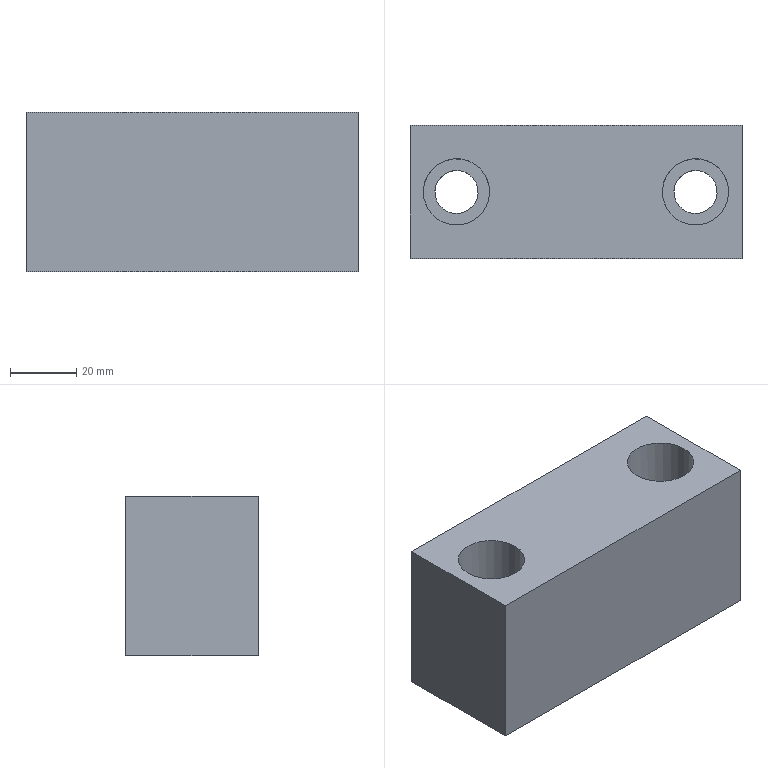Part | STEP file | gslz 2016.10.28-13_id774_x_t | 1 solid | 12 faces | box 100 x 40 x 48 mm | volume 169823 mm3 | plane 8 | cylinder 4 | commonest cylinder face diameters 13 x2 20 x2
STEP:
#1=CARTESIAN_POINT('',(0.,0.,0.));
#2=DIRECTION('',(0.,0.,1.));
#3=DIRECTION('',(1.,0.,0.));
#4=AXIS2_PLACEMENT_3D('',#1,#2,#3);
#5=CARTESIAN_POINT('',(-1056.695,-13.439,0.));
#6=VERTEX_POINT('',#5);
#7=CARTESIAN_POINT('',(-1156.695,-13.439,0.));
#8=VERTEX_POINT('',#7);
#9=CARTESIAN_POINT('',(-1172.695,-13.439,0.));
#10=DIRECTION('',(-1.,0.,0.));
#11=VECTOR('',#10,1.);
#12=LINE('',#9,#11);
#13=CARTESIAN_POINT('',(-1056.695,-13.439,-43.));
#14=DIRECTION('',(0.,1.,0.));
#15=DIRECTION('',(-1.,0.,0.));
#16=AXIS2_PLACEMENT_3D('',#13,#14,#15);
#17=PLANE('',#16);
#18=CARTESIAN_POINT('',(116.,43.));
#19=DIRECTION('',(1.,0.));
#20=VECTOR('',#19,1.);
#21=LINE('',#18,#20);
#22=(GEOMETRIC_REPRESENTATION_CONTEXT(2)PARAMETRIC_REPRESENTATION_CONTEXT()REPRESENTATION_CONTEXT('',''));
#23=DEFINITIONAL_REPRESENTATION('',(#21),#22);
#24=PCURVE('',#17,#23);
#25=CARTESIAN_POINT('',(-1172.695,-123.667,0.));
#26=DIRECTION('',(0.,0.,1.));
#27=DIRECTION('',(-1.,0.,0.));
#28=AXIS2_PLACEMENT_3D('',#25,#26,#27);
#29=PLANE('',#28);
#30=CARTESIAN_POINT('',(0.,-110.228));
#31=DIRECTION('',(1.,0.));
#32=VECTOR('',#31,1.);
#33=LINE('',#30,#32);
#34=(GEOMETRIC_REPRESENTATION_CONTEXT(2)PARAMETRIC_REPRESENTATION_CONTEXT()REPRESENTATION_CONTEXT('',''));
#35=DEFINITIONAL_REPRESENTATION('',(#33),#34);
#36=PCURVE('',#29,#35);
#37=SURFACE_CURVE('',#12,(#24,#36),.PCURVE_S1.);
#38=EDGE_CURVE('',#6,#8,#37,.T.);
#39=ORIENTED_EDGE('',*,*,#38,.F.);
#40=CARTESIAN_POINT('',(-1056.695,-13.439,-48.));
#41=VERTEX_POINT('',#40);
#42=CARTESIAN_POINT('',(-1056.695,-13.439,-43.));
#43=DIRECTION('',(0.,0.,1.));
#44=VECTOR('',#43,1.);
#45=LINE('',#42,#44);
#46=CARTESIAN_POINT('',(0.,0.));
#47=DIRECTION('',(0.,1.));
#48=VECTOR('',#47,1.);
#49=LINE('',#46,#48);
#50=(GEOMETRIC_REPRESENTATION_CONTEXT(2)PARAMETRIC_REPRESENTATION_CONTEXT()REPRESENTATION_CONTEXT('',''));
#51=DEFINITIONAL_REPRESENTATION('',(#49),#50);
#52=PCURVE('',#17,#51);
#53=CARTESIAN_POINT('',(-1056.695,-214.939,-43.));
#54=DIRECTION('',(1.,0.,0.));
#55=DIRECTION('',(0.,0.,1.));
#56=AXIS2_PLACEMENT_3D('',#53,#54,#55);
#57=PLANE('',#56);
#58=CARTESIAN_POINT('',(0.,-201.5));
#59=DIRECTION('',(1.,0.));
#60=VECTOR('',#59,1.);
#61=LINE('',#58,#60);
#62=(GEOMETRIC_REPRESENTATION_CONTEXT(2)PARAMETRIC_REPRESENTATION_CONTEXT()REPRESENTATION_CONTEXT('',''));
#63=DEFINITIONAL_REPRESENTATION('',(#61),#62);
#64=PCURVE('',#57,#63);
#65=SURFACE_CURVE('',#45,(#52,#64),.PCURVE_S1.);
#66=EDGE_CURVE('',#41,#6,#65,.T.);
#67=ORIENTED_EDGE('',*,*,#66,.F.);
#68=CARTESIAN_POINT('',(-1156.695,-13.439,-48.));
#69=VERTEX_POINT('',#68);
#70=CARTESIAN_POINT('',(-1119.195,-13.439,-48.));
#71=DIRECTION('',(-1.,0.,0.));
#72=VECTOR('',#71,1.);
#73=LINE('',#70,#72);
#74=CARTESIAN_POINT('',(62.5,-5.));
#75=DIRECTION('',(1.,0.));
#76=VECTOR('',#75,1.);
#77=LINE('',#74,#76);
#78=(GEOMETRIC_REPRESENTATION_CONTEXT(2)PARAMETRIC_REPRESENTATION_CONTEXT()REPRESENTATION_CONTEXT('',''));
#79=DEFINITIONAL_REPRESENTATION('',(#77),#78);
#80=PCURVE('',#17,#79);
#81=CARTESIAN_POINT('',(-1119.195,-219.939,-48.));
#82=DIRECTION('',(0.,0.,1.));
#83=DIRECTION('',(-1.,0.,0.));
#84=AXIS2_PLACEMENT_3D('',#81,#82,#83);
#85=PLANE('',#84);
#86=CARTESIAN_POINT('',(0.,-206.5));
#87=DIRECTION('',(1.,0.));
#88=VECTOR('',#87,1.);
#89=LINE('',#86,#88);
#90=(GEOMETRIC_REPRESENTATION_CONTEXT(2)PARAMETRIC_REPRESENTATION_CONTEXT()REPRESENTATION_CONTEXT('',''));
#91=DEFINITIONAL_REPRESENTATION('',(#89),#90);
#92=PCURVE('',#85,#91);
#93=SURFACE_CURVE('',#73,(#80,#92),.PCURVE_S1.);
#94=EDGE_CURVE('',#41,#69,#93,.T.);
#95=ORIENTED_EDGE('',*,*,#94,.T.);
#96=CARTESIAN_POINT('',(-1156.695,-13.439,-43.));
#97=DIRECTION('',(0.,0.,1.));
#98=VECTOR('',#97,1.);
#99=LINE('',#96,#98);
#100=CARTESIAN_POINT('',(100.,0.));
#101=DIRECTION('',(0.,1.));
#102=VECTOR('',#101,1.);
#103=LINE('',#100,#102);
#104=(GEOMETRIC_REPRESENTATION_CONTEXT(2)PARAMETRIC_REPRESENTATION_CONTEXT()REPRESENTATION_CONTEXT('',''));
#105=DEFINITIONAL_REPRESENTATION('',(#103),#104);
#106=PCURVE('',#17,#105);
#107=CARTESIAN_POINT('',(-1156.695,-24.939,-43.));
#108=DIRECTION('',(-1.,0.,0.));
#109=DIRECTION('',(0.,-1.,0.));
#110=AXIS2_PLACEMENT_3D('',#107,#108,#109);
#111=PLANE('',#110);
#112=CARTESIAN_POINT('',(-11.5,0.));
#113=DIRECTION('',(0.,1.));
#114=VECTOR('',#113,1.);
#115=LINE('',#112,#114);
#116=(GEOMETRIC_REPRESENTATION_CONTEXT(2)PARAMETRIC_REPRESENTATION_CONTEXT()REPRESENTATION_CONTEXT('',''));
#117=DEFINITIONAL_REPRESENTATION('',(#115),#116);
#118=PCURVE('',#111,#117);
#119=SURFACE_CURVE('',#99,(#106,#118),.PCURVE_S1.);
#120=EDGE_CURVE('',#69,#8,#119,.T.);
#121=ORIENTED_EDGE('',*,*,#120,.T.);
#122=EDGE_LOOP('',(#39,#67,#95,#121));
#123=FACE_BOUND('',#122,.T.);
#124=ADVANCED_FACE('',(#123),#17,.T.);
#125=CARTESIAN_POINT('',(-1156.695,-53.439,0.));
#126=VERTEX_POINT('',#125);
#127=CARTESIAN_POINT('',(-1156.695,-24.939,0.));
#128=DIRECTION('',(0.,-1.,0.));
#129=VECTOR('',#128,1.);
#130=LINE('',#127,#129);
#131=CARTESIAN_POINT('',(0.,43.));
#132=DIRECTION('',(1.,0.));
#133=VECTOR('',#132,1.);
#134=LINE('',#131,#133);
#135=(GEOMETRIC_REPRESENTATION_CONTEXT(2)PARAMETRIC_REPRESENTATION_CONTEXT()REPRESENTATION_CONTEXT('',''));
#136=DEFINITIONAL_REPRESENTATION('',(#134),#135);
#137=PCURVE('',#111,#136);
#138=CARTESIAN_POINT('',(-16.,-98.728));
#139=DIRECTION('',(0.,1.));
#140=VECTOR('',#139,1.);
#141=LINE('',#138,#140);
#142=(GEOMETRIC_REPRESENTATION_CONTEXT(2)PARAMETRIC_REPRESENTATION_CONTEXT()REPRESENTATION_CONTEXT('',''));
#143=DEFINITIONAL_REPRESENTATION('',(#141),#142);
#144=PCURVE('',#29,#143);
#145=SURFACE_CURVE('',#130,(#137,#144),.PCURVE_S1.);
#146=EDGE_CURVE('',#8,#126,#145,.T.);
#147=ORIENTED_EDGE('',*,*,#146,.F.);
#148=ORIENTED_EDGE('',*,*,#120,.F.);
#149=CARTESIAN_POINT('',(-1156.695,-53.439,-48.));
#150=VERTEX_POINT('',#149);
#151=CARTESIAN_POINT('',(-1156.695,-219.939,-48.));
#152=DIRECTION('',(0.,-1.,0.));
#153=VECTOR('',#152,1.);
#154=LINE('',#151,#153);
#155=CARTESIAN_POINT('',(195.,-5.));
#156=DIRECTION('',(1.,0.));
#157=VECTOR('',#156,1.);
#158=LINE('',#155,#157);
#159=(GEOMETRIC_REPRESENTATION_CONTEXT(2)PARAMETRIC_REPRESENTATION_CONTEXT()REPRESENTATION_CONTEXT('',''));
#160=DEFINITIONAL_REPRESENTATION('',(#158),#159);
#161=PCURVE('',#111,#160);
#162=CARTESIAN_POINT('',(37.5,0.));
#163=DIRECTION('',(0.,1.));
#164=VECTOR('',#163,1.);
#165=LINE('',#162,#164);
#166=(GEOMETRIC_REPRESENTATION_CONTEXT(2)PARAMETRIC_REPRESENTATION_CONTEXT()REPRESENTATION_CONTEXT('',''));
#167=DEFINITIONAL_REPRESENTATION('',(#165),#166);
#168=PCURVE('',#85,#167);
#169=SURFACE_CURVE('',#154,(#161,#168),.PCURVE_S1.);
#170=EDGE_CURVE('',#69,#150,#169,.T.);
#171=ORIENTED_EDGE('',*,*,#170,.T.);
#172=CARTESIAN_POINT('',(-1156.695,-53.439,-25.5));
#173=DIRECTION('',(0.,0.,-1.));
#174=VECTOR('',#173,1.);
#175=LINE('',#172,#174);
#176=CARTESIAN_POINT('',(28.5,17.5));
#177=DIRECTION('',(0.,-1.));
#178=VECTOR('',#177,1.);
#179=LINE('',#176,#178);
#180=(GEOMETRIC_REPRESENTATION_CONTEXT(2)PARAMETRIC_REPRESENTATION_CONTEXT()REPRESENTATION_CONTEXT('',''));
#181=DEFINITIONAL_REPRESENTATION('',(#179),#180);
#182=PCURVE('',#111,#181);
#183=CARTESIAN_POINT('',(-1101.695,-53.439,-25.5));
#184=DIRECTION('',(0.,1.,0.));
#185=DIRECTION('',(0.,0.,-1.));
#186=AXIS2_PLACEMENT_3D('',#183,#184,#185);
#187=PLANE('',#186);
#188=CARTESIAN_POINT('',(0.,55.));
#189=DIRECTION('',(1.,0.));
#190=VECTOR('',#189,1.);
#191=LINE('',#188,#190);
#192=(GEOMETRIC_REPRESENTATION_CONTEXT(2)PARAMETRIC_REPRESENTATION_CONTEXT()REPRESENTATION_CONTEXT('',''));
#193=DEFINITIONAL_REPRESENTATION('',(#191),#192);
#194=PCURVE('',#187,#193);
#195=SURFACE_CURVE('',#175,(#182,#194),.PCURVE_S1.);
#196=EDGE_CURVE('',#126,#150,#195,.T.);
#197=ORIENTED_EDGE('',*,*,#196,.F.);
#198=EDGE_LOOP('',(#147,#148,#171,#197));
#199=FACE_BOUND('',#198,.T.);
#200=ADVANCED_FACE('',(#199),#111,.T.);
#201=ORIENTED_EDGE('',*,*,#196,.T.);
#202=CARTESIAN_POINT('',(-1056.695,-53.439,-48.));
#203=VERTEX_POINT('',#202);
#204=CARTESIAN_POINT('',(-1119.195,-53.439,-48.));
#205=DIRECTION('',(1.,0.,0.));
#206=VECTOR('',#205,1.);
#207=LINE('',#204,#206);
#208=CARTESIAN_POINT('',(22.5,17.5));
#209=DIRECTION('',(0.,-1.));
#210=VECTOR('',#209,1.);
#211=LINE('',#208,#210);
#212=(GEOMETRIC_REPRESENTATION_CONTEXT(2)PARAMETRIC_REPRESENTATION_CONTEXT()REPRESENTATION_CONTEXT('',''));
#213=DEFINITIONAL_REPRESENTATION('',(#211),#212);
#214=PCURVE('',#187,#213);
#215=CARTESIAN_POINT('',(0.,-166.5));
#216=DIRECTION('',(-1.,0.));
#217=VECTOR('',#216,1.);
#218=LINE('',#215,#217);
#219=(GEOMETRIC_REPRESENTATION_CONTEXT(2)PARAMETRIC_REPRESENTATION_CONTEXT()REPRESENTATION_CONTEXT('',''));
#220=DEFINITIONAL_REPRESENTATION('',(#218),#219);
#221=PCURVE('',#85,#220);
#222=SURFACE_CURVE('',#207,(#214,#221),.PCURVE_S1.);
#223=EDGE_CURVE('',#150,#203,#222,.T.);
#224=ORIENTED_EDGE('',*,*,#223,.T.);
#225=CARTESIAN_POINT('',(-1056.695,-53.439,0.));
#226=VERTEX_POINT('',#225);
#227=CARTESIAN_POINT('',(-1056.695,-53.439,-43.));
#228=DIRECTION('',(0.,0.,-1.));
#229=VECTOR('',#228,1.);
#230=LINE('',#227,#229);
#231=CARTESIAN_POINT('',(17.5,-45.));
#232=DIRECTION('',(1.,0.));
#233=VECTOR('',#232,1.);
#234=LINE('',#231,#233);
#235=(GEOMETRIC_REPRESENTATION_CONTEXT(2)PARAMETRIC_REPRESENTATION_CONTEXT()REPRESENTATION_CONTEXT('',''));
#236=DEFINITIONAL_REPRESENTATION('',(#234),#235);
#237=PCURVE('',#187,#236);
#238=CARTESIAN_POINT('',(0.,-161.5));
#239=DIRECTION('',(-1.,0.));
#240=VECTOR('',#239,1.);
#241=LINE('',#238,#240);
#242=(GEOMETRIC_REPRESENTATION_CONTEXT(2)PARAMETRIC_REPRESENTATION_CONTEXT()REPRESENTATION_CONTEXT('',''));
#243=DEFINITIONAL_REPRESENTATION('',(#241),#242);
#244=PCURVE('',#57,#243);
#245=SURFACE_CURVE('',#230,(#237,#244),.PCURVE_S1.);
#246=EDGE_CURVE('',#226,#203,#245,.T.);
#247=ORIENTED_EDGE('',*,*,#246,.F.);
#248=CARTESIAN_POINT('',(-1101.695,-53.439,0.));
#249=DIRECTION('',(-1.,0.,0.));
#250=VECTOR('',#249,1.);
#251=LINE('',#248,#250);
#252=CARTESIAN_POINT('',(-25.5,0.));
#253=DIRECTION('',(0.,1.));
#254=VECTOR('',#253,1.);
#255=LINE('',#252,#254);
#256=(GEOMETRIC_REPRESENTATION_CONTEXT(2)PARAMETRIC_REPRESENTATION_CONTEXT()REPRESENTATION_CONTEXT('',''));
#257=DEFINITIONAL_REPRESENTATION('',(#255),#256);
#258=PCURVE('',#187,#257);
#259=CARTESIAN_POINT('',(-71.,-70.228));
#260=DIRECTION('',(1.,0.));
#261=VECTOR('',#260,1.);
#262=LINE('',#259,#261);
#263=(GEOMETRIC_REPRESENTATION_CONTEXT(2)PARAMETRIC_REPRESENTATION_CONTEXT()REPRESENTATION_CONTEXT('',''));
#264=DEFINITIONAL_REPRESENTATION('',(#262),#263);
#265=PCURVE('',#29,#264);
#266=SURFACE_CURVE('',#251,(#258,#265),.PCURVE_S1.);
#267=EDGE_CURVE('',#226,#126,#266,.T.);
#268=ORIENTED_EDGE('',*,*,#267,.T.);
#269=EDGE_LOOP('',(#201,#224,#247,#268));
#270=FACE_BOUND('',#269,.T.);
#271=ADVANCED_FACE('',(#270),#187,.F.);
#272=ORIENTED_EDGE('',*,*,#246,.T.);
#273=CARTESIAN_POINT('',(-1056.695,-219.939,-48.));
#274=DIRECTION('',(0.,1.,0.));
#275=VECTOR('',#274,1.);
#276=LINE('',#273,#275);
#277=CARTESIAN_POINT('',(-5.,5.));
#278=DIRECTION('',(0.,-1.));
#279=VECTOR('',#278,1.);
#280=LINE('',#277,#279);
#281=(GEOMETRIC_REPRESENTATION_CONTEXT(2)PARAMETRIC_REPRESENTATION_CONTEXT()REPRESENTATION_CONTEXT('',''));
#282=DEFINITIONAL_REPRESENTATION('',(#280),#281);
#283=PCURVE('',#57,#282);
#284=CARTESIAN_POINT('',(-62.5,0.));
#285=DIRECTION('',(0.,-1.));
#286=VECTOR('',#285,1.);
#287=LINE('',#284,#286);
#288=(GEOMETRIC_REPRESENTATION_CONTEXT(2)PARAMETRIC_REPRESENTATION_CONTEXT()REPRESENTATION_CONTEXT('',''));
#289=DEFINITIONAL_REPRESENTATION('',(#287),#288);
#290=PCURVE('',#85,#289);
#291=SURFACE_CURVE('',#276,(#283,#290),.PCURVE_S1.);
#292=EDGE_CURVE('',#203,#41,#291,.T.);
#293=ORIENTED_EDGE('',*,*,#292,.T.);
#294=ORIENTED_EDGE('',*,*,#66,.T.);
#295=CARTESIAN_POINT('',(-1056.695,-214.939,0.));
#296=DIRECTION('',(0.,1.,0.));
#297=VECTOR('',#296,1.);
#298=LINE('',#295,#297);
#299=CARTESIAN_POINT('',(43.,0.));
#300=DIRECTION('',(0.,-1.));
#301=VECTOR('',#300,1.);
#302=LINE('',#299,#301);
#303=(GEOMETRIC_REPRESENTATION_CONTEXT(2)PARAMETRIC_REPRESENTATION_CONTEXT()REPRESENTATION_CONTEXT('',''));
#304=DEFINITIONAL_REPRESENTATION('',(#302),#303);
#305=PCURVE('',#57,#304);
#306=CARTESIAN_POINT('',(-116.,91.272));
#307=DIRECTION('',(0.,-1.));
#308=VECTOR('',#307,1.);
#309=LINE('',#306,#308);
#310=(GEOMETRIC_REPRESENTATION_CONTEXT(2)PARAMETRIC_REPRESENTATION_CONTEXT()REPRESENTATION_CONTEXT('',''));
#311=DEFINITIONAL_REPRESENTATION('',(#309),#310);
#312=PCURVE('',#29,#311);
#313=SURFACE_CURVE('',#298,(#305,#312),.PCURVE_S1.);
#314=EDGE_CURVE('',#226,#6,#313,.T.);
#315=ORIENTED_EDGE('',*,*,#314,.F.);
#316=EDGE_LOOP('',(#272,#293,#294,#315));
#317=FACE_BOUND('',#316,.T.);
#318=ADVANCED_FACE('',(#317),#57,.T.);
#319=CARTESIAN_POINT('',(-1071.786,-39.847,-48.));
#320=VERTEX_POINT('',#319);
#321=CARTESIAN_POINT('',(-1070.695,-33.439,-48.));
#322=DIRECTION('',(0.,0.,1.));
#323=DIRECTION('',(-0.1678,-0.9858,0.));
#324=AXIS2_PLACEMENT_3D('',#321,#322,#323);
#325=CIRCLE('',#324,6.5);
#326=CARTESIAN_POINT('',(-48.5,-186.5));
#327=DIRECTION('',(0.1678,0.9858));
#328=AXIS2_PLACEMENT_2D('',#326,#327);
#329=CIRCLE('',#328,6.5);
#330=(GEOMETRIC_REPRESENTATION_CONTEXT(2)PARAMETRIC_REPRESENTATION_CONTEXT()REPRESENTATION_CONTEXT('',''));
#331=DEFINITIONAL_REPRESENTATION('',(#329),#330);
#332=PCURVE('',#85,#331);
#333=CARTESIAN_POINT('',(-1070.695,-33.439,-8.541));
#334=DIRECTION('',(0.,0.,-1.));
#335=DIRECTION('',(-1.,0.,0.));
#336=AXIS2_PLACEMENT_3D('',#333,#334,#335);
#337=CYLINDRICAL_SURFACE('',#336,6.5);
#338=CARTESIAN_POINT('',(11.164,39.459));
#339=DIRECTION('',(-1.,0.));
#340=VECTOR('',#339,1.);
#341=LINE('',#338,#340);
#342=(GEOMETRIC_REPRESENTATION_CONTEXT(2)PARAMETRIC_REPRESENTATION_CONTEXT()REPRESENTATION_CONTEXT('',''));
#343=DEFINITIONAL_REPRESENTATION('',(#341),#342);
#344=PCURVE('',#337,#343);
#345=SURFACE_CURVE('',#325,(#332,#344),.PCURVE_S1.);
#346=EDGE_CURVE('',#320,#320,#345,.T.);
#347=ORIENTED_EDGE('',*,*,#346,.T.);
#348=EDGE_LOOP('',(#347));
#349=FACE_BOUND('',#348,.T.);
#350=CARTESIAN_POINT('',(-1143.786,-39.847,-48.));
#351=VERTEX_POINT('',#350);
#352=CARTESIAN_POINT('',(-1142.695,-33.439,-48.));
#353=DIRECTION('',(0.,0.,1.));
#354=DIRECTION('',(-0.1678,-0.9858,0.));
#355=AXIS2_PLACEMENT_3D('',#352,#353,#354);
#356=CIRCLE('',#355,6.5);
#357=CARTESIAN_POINT('',(23.5,-186.5));
#358=DIRECTION('',(0.1678,0.9858));
#359=AXIS2_PLACEMENT_2D('',#357,#358);
#360=CIRCLE('',#359,6.5);
#361=(GEOMETRIC_REPRESENTATION_CONTEXT(2)PARAMETRIC_REPRESENTATION_CONTEXT()REPRESENTATION_CONTEXT('',''));
#362=DEFINITIONAL_REPRESENTATION('',(#360),#361);
#363=PCURVE('',#85,#362);
#364=CARTESIAN_POINT('',(-1142.695,-33.439,-8.541));
#365=DIRECTION('',(0.,0.,-1.));
#366=DIRECTION('',(-1.,0.,0.));
#367=AXIS2_PLACEMENT_3D('',#364,#365,#366);
#368=CYLINDRICAL_SURFACE('',#367,6.5);
#369=CARTESIAN_POINT('',(11.164,39.459));
#370=DIRECTION('',(-1.,0.));
#371=VECTOR('',#370,1.);
#372=LINE('',#369,#371);
#373=(GEOMETRIC_REPRESENTATION_CONTEXT(2)PARAMETRIC_REPRESENTATION_CONTEXT()REPRESENTATION_CONTEXT('',''));
#374=DEFINITIONAL_REPRESENTATION('',(#372),#373);
#375=PCURVE('',#368,#374);
#376=SURFACE_CURVE('',#356,(#363,#375),.PCURVE_S1.);
#377=EDGE_CURVE('',#351,#351,#376,.T.);
#378=ORIENTED_EDGE('',*,*,#377,.T.);
#379=EDGE_LOOP('',(#378));
#380=FACE_BOUND('',#379,.T.);
#381=ORIENTED_EDGE('',*,*,#292,.F.);
#382=ORIENTED_EDGE('',*,*,#223,.F.);
#383=ORIENTED_EDGE('',*,*,#170,.F.);
#384=ORIENTED_EDGE('',*,*,#94,.F.);
#385=EDGE_LOOP('',(#381,#382,#383,#384));
#386=FACE_BOUND('',#385,.T.);
#387=ADVANCED_FACE('',(#349,#380,#386),#85,.F.);
#388=CARTESIAN_POINT('',(-1060.695,-33.439,0.));
#389=VERTEX_POINT('',#388);
#390=CARTESIAN_POINT('',(-1072.373,-43.297,0.));
#391=VERTEX_POINT('',#390);
#392=CARTESIAN_POINT('',(-1070.695,-33.439,0.));
#393=DIRECTION('',(0.,0.,1.));
#394=DIRECTION('',(1.,0.,0.));
#395=AXIS2_PLACEMENT_3D('',#392,#393,#394);
#396=CIRCLE('',#395,10.);
#397=CARTESIAN_POINT('',(-102.,-90.228));
#398=DIRECTION('',(-1.,0.));
#399=AXIS2_PLACEMENT_2D('',#397,#398);
#400=CIRCLE('',#399,10.);
#401=(GEOMETRIC_REPRESENTATION_CONTEXT(2)PARAMETRIC_REPRESENTATION_CONTEXT()REPRESENTATION_CONTEXT('',''));
#402=DEFINITIONAL_REPRESENTATION('',(#400),#401);
#403=PCURVE('',#29,#402);
#404=CARTESIAN_POINT('',(-1070.695,-33.439,-8.541));
#405=DIRECTION('',(0.,0.,-1.));
#406=DIRECTION('',(-1.,0.,0.));
#407=AXIS2_PLACEMENT_3D('',#404,#405,#406);
#408=CYLINDRICAL_SURFACE('',#407,10.);
#409=CARTESIAN_POINT('',(9.425,-8.541));
#410=DIRECTION('',(-1.,0.));
#411=VECTOR('',#410,1.);
#412=LINE('',#409,#411);
#413=(GEOMETRIC_REPRESENTATION_CONTEXT(2)PARAMETRIC_REPRESENTATION_CONTEXT()REPRESENTATION_CONTEXT('',''));
#414=DEFINITIONAL_REPRESENTATION('',(#412),#413);
#415=PCURVE('',#408,#414);
#416=SURFACE_CURVE('',#396,(#403,#415),.PCURVE_S1.);
#417=EDGE_CURVE('',#389,#391,#416,.T.);
#418=ORIENTED_EDGE('',*,*,#417,.F.);
#419=CARTESIAN_POINT('',(-1070.695,-33.439,0.));
#420=DIRECTION('',(0.,0.,1.));
#421=DIRECTION('',(1.,0.,0.));
#422=AXIS2_PLACEMENT_3D('',#419,#420,#421);
#423=CIRCLE('',#422,10.);
#424=CARTESIAN_POINT('',(-102.,-90.228));
#425=DIRECTION('',(-1.,0.));
#426=AXIS2_PLACEMENT_2D('',#424,#425);
#427=CIRCLE('',#426,10.);
#428=(GEOMETRIC_REPRESENTATION_CONTEXT(2)PARAMETRIC_REPRESENTATION_CONTEXT()REPRESENTATION_CONTEXT('',''));
#429=DEFINITIONAL_REPRESENTATION('',(#427),#428);
#430=PCURVE('',#29,#429);
#431=CARTESIAN_POINT('',(15.708,-8.541));
#432=DIRECTION('',(-1.,0.));
#433=VECTOR('',#432,1.);
#434=LINE('',#431,#433);
#435=(GEOMETRIC_REPRESENTATION_CONTEXT(2)PARAMETRIC_REPRESENTATION_CONTEXT()REPRESENTATION_CONTEXT('',''));
#436=DEFINITIONAL_REPRESENTATION('',(#434),#435);
#437=PCURVE('',#408,#436);
#438=SURFACE_CURVE('',#423,(#430,#437),.PCURVE_S1.);
#439=EDGE_CURVE('',#391,#389,#438,.T.);
#440=ORIENTED_EDGE('',*,*,#439,.F.);
#441=EDGE_LOOP('',(#418,#440));
#442=FACE_BOUND('',#441,.T.);
#443=CARTESIAN_POINT('',(-1132.695,-33.439,0.));
#444=VERTEX_POINT('',#443);
#445=CARTESIAN_POINT('',(-1144.373,-43.297,0.));
#446=VERTEX_POINT('',#445);
#447=CARTESIAN_POINT('',(-1142.695,-33.439,0.));
#448=DIRECTION('',(0.,0.,1.));
#449=DIRECTION('',(1.,0.,0.));
#450=AXIS2_PLACEMENT_3D('',#447,#448,#449);
#451=CIRCLE('',#450,10.);
#452=CARTESIAN_POINT('',(-30.,-90.228));
#453=DIRECTION('',(-1.,0.));
#454=AXIS2_PLACEMENT_2D('',#452,#453);
#455=CIRCLE('',#454,10.);
#456=(GEOMETRIC_REPRESENTATION_CONTEXT(2)PARAMETRIC_REPRESENTATION_CONTEXT()REPRESENTATION_CONTEXT('',''));
#457=DEFINITIONAL_REPRESENTATION('',(#455),#456);
#458=PCURVE('',#29,#457);
#459=CARTESIAN_POINT('',(-1142.695,-33.439,-8.541));
#460=DIRECTION('',(0.,0.,-1.));
#461=DIRECTION('',(-1.,0.,0.));
#462=AXIS2_PLACEMENT_3D('',#459,#460,#461);
#463=CYLINDRICAL_SURFACE('',#462,10.);
#464=CARTESIAN_POINT('',(9.425,-8.541));
#465=DIRECTION('',(-1.,0.));
#466=VECTOR('',#465,1.);
#467=LINE('',#464,#466);
#468=(GEOMETRIC_REPRESENTATION_CONTEXT(2)PARAMETRIC_REPRESENTATION_CONTEXT()REPRESENTATION_CONTEXT('',''));
#469=DEFINITIONAL_REPRESENTATION('',(#467),#468);
#470=PCURVE('',#463,#469);
#471=SURFACE_CURVE('',#451,(#458,#470),.PCURVE_S1.);
#472=EDGE_CURVE('',#444,#446,#471,.T.);
#473=ORIENTED_EDGE('',*,*,#472,.F.);
#474=CARTESIAN_POINT('',(-1142.695,-33.439,0.));
#475=DIRECTION('',(0.,0.,1.));
#476=DIRECTION('',(1.,0.,0.));
#477=AXIS2_PLACEMENT_3D('',#474,#475,#476);
#478=CIRCLE('',#477,10.);
#479=CARTESIAN_POINT('',(-30.,-90.228));
#480=DIRECTION('',(-1.,0.));
#481=AXIS2_PLACEMENT_2D('',#479,#480);
#482=CIRCLE('',#481,10.);
#483=(GEOMETRIC_REPRESENTATION_CONTEXT(2)PARAMETRIC_REPRESENTATION_CONTEXT()REPRESENTATION_CONTEXT('',''));
#484=DEFINITIONAL_REPRESENTATION('',(#482),#483);
#485=PCURVE('',#29,#484);
#486=CARTESIAN_POINT('',(15.708,-8.541));
#487=DIRECTION('',(-1.,0.));
#488=VECTOR('',#487,1.);
#489=LINE('',#486,#488);
#490=(GEOMETRIC_REPRESENTATION_CONTEXT(2)PARAMETRIC_REPRESENTATION_CONTEXT()REPRESENTATION_CONTEXT('',''));
#491=DEFINITIONAL_REPRESENTATION('',(#489),#490);
#492=PCURVE('',#463,#491);
#493=SURFACE_CURVE('',#478,(#485,#492),.PCURVE_S1.);
#494=EDGE_CURVE('',#446,#444,#493,.T.);
#495=ORIENTED_EDGE('',*,*,#494,.F.);
#496=EDGE_LOOP('',(#473,#495));
#497=FACE_BOUND('',#496,.T.);
#498=ORIENTED_EDGE('',*,*,#267,.F.);
#499=ORIENTED_EDGE('',*,*,#314,.T.);
#500=ORIENTED_EDGE('',*,*,#38,.T.);
#501=ORIENTED_EDGE('',*,*,#146,.T.);
#502=EDGE_LOOP('',(#498,#499,#500,#501));
#503=FACE_BOUND('',#502,.T.);
#504=ADVANCED_FACE('',(#442,#497,#503),#29,.T.);
#505=CARTESIAN_POINT('',(-1143.786,-39.847,-26.));
#506=VERTEX_POINT('',#505);
#507=CARTESIAN_POINT('',(-1142.695,-33.439,-26.));
#508=DIRECTION('',(0.,0.,1.));
#509=DIRECTION('',(-0.1678,-0.9858,0.));
#510=AXIS2_PLACEMENT_3D('',#507,#508,#509);
#511=CIRCLE('',#510,6.5);
#512=CARTESIAN_POINT('',(-1142.695,-33.439,-26.));
#513=DIRECTION('',(0.,0.,1.));
#514=DIRECTION('',(-0.1678,-0.9858,0.));
#515=AXIS2_PLACEMENT_3D('',#512,#513,#514);
#516=PLANE('',#515);
#517=CARTESIAN_POINT('',(0.,0.));
#518=DIRECTION('',(1.,0.));
#519=AXIS2_PLACEMENT_2D('',#517,#518);
#520=CIRCLE('',#519,6.5);
#521=(GEOMETRIC_REPRESENTATION_CONTEXT(2)PARAMETRIC_REPRESENTATION_CONTEXT()REPRESENTATION_CONTEXT('',''));
#522=DEFINITIONAL_REPRESENTATION('',(#520),#521);
#523=PCURVE('',#516,#522);
#524=CARTESIAN_POINT('',(11.164,17.459));
#525=DIRECTION('',(-1.,0.));
#526=VECTOR('',#525,1.);
#527=LINE('',#524,#526);
#528=(GEOMETRIC_REPRESENTATION_CONTEXT(2)PARAMETRIC_REPRESENTATION_CONTEXT()REPRESENTATION_CONTEXT('',''));
#529=DEFINITIONAL_REPRESENTATION('',(#527),#528);
#530=PCURVE('',#368,#529);
#531=SURFACE_CURVE('',#511,(#523,#530),.PCURVE_S1.);
#532=EDGE_CURVE('',#506,#506,#531,.T.);
#533=ORIENTED_EDGE('',*,*,#532,.F.);
#534=EDGE_LOOP('',(#533));
#535=FACE_BOUND('',#534,.T.);
#536=CARTESIAN_POINT('',(-1144.373,-43.297,-26.));
#537=VERTEX_POINT('',#536);
#538=CARTESIAN_POINT('',(-1142.695,-33.439,-26.));
#539=DIRECTION('',(0.,0.,-1.));
#540=DIRECTION('',(-0.1678,-0.9858,0.));
#541=AXIS2_PLACEMENT_3D('',#538,#539,#540);
#542=CIRCLE('',#541,10.);
#543=CARTESIAN_POINT('',(10.,0.));
#544=CARTESIAN_POINT('',(10.,-17.321));
#545=CARTESIAN_POINT('',(-5.,-8.66));
#546=CARTESIAN_POINT('',(-20.,0.));
#547=CARTESIAN_POINT('',(-5.,8.66));
#548=CARTESIAN_POINT('',(10.,17.321));
#549=CARTESIAN_POINT('',(10.,0.));
#550=(BOUNDED_CURVE()B_SPLINE_CURVE(2,(#543,#544,#545,#546,#547,#548,#549),.UNSPECIFIED.,.T.,.F.)B_SPLINE_CURVE_WITH_KNOTS((1,2,2,2,2,1),(-2.094,0.,2.094,4.189,6.283,8.378),.UNSPECIFIED.)CURVE()GEOMETRIC_REPRESENTATION_ITEM()RATIONAL_B_SPLINE_CURVE((1.,0.5,1.,0.5,1.,0.5,1.))REPRESENTATION_ITEM(''));
#551=(GEOMETRIC_REPRESENTATION_CONTEXT(2)PARAMETRIC_REPRESENTATION_CONTEXT()REPRESENTATION_CONTEXT('',''));
#552=DEFINITIONAL_REPRESENTATION('',(#550),#551);
#553=PCURVE('',#516,#552);
#554=CARTESIAN_POINT('',(4.881,17.459));
#555=DIRECTION('',(1.,0.));
#556=VECTOR('',#555,1.);
#557=LINE('',#554,#556);
#558=(GEOMETRIC_REPRESENTATION_CONTEXT(2)PARAMETRIC_REPRESENTATION_CONTEXT()REPRESENTATION_CONTEXT('',''));
#559=DEFINITIONAL_REPRESENTATION('',(#557),#558);
#560=PCURVE('',#463,#559);
#561=SURFACE_CURVE('',#542,(#553,#560),.PCURVE_S1.);
#562=EDGE_CURVE('',#537,#537,#561,.T.);
#563=ORIENTED_EDGE('',*,*,#562,.F.);
#564=EDGE_LOOP('',(#563));
#565=FACE_BOUND('',#564,.T.);
#566=ADVANCED_FACE('',(#535,#565),#516,.T.);
#567=ORIENTED_EDGE('',*,*,#494,.F.);
#568=CARTESIAN_POINT('',(-1144.373,-43.297,0.));
#569=CARTESIAN_POINT('',(-1144.373,-43.297,-26.));
#570=B_SPLINE_CURVE_WITH_KNOTS('',1,(#568,#569),.UNSPECIFIED.,.F.,.F.,(2,2),(-8.541,17.459),.PIECEWISE_BEZIER_KNOTS.);
#571=CARTESIAN_POINT('',(11.164,0.));
#572=DIRECTION('',(0.,1.));
#573=VECTOR('',#572,1.);
#574=LINE('',#571,#573);
#575=(GEOMETRIC_REPRESENTATION_CONTEXT(2)PARAMETRIC_REPRESENTATION_CONTEXT()REPRESENTATION_CONTEXT('',''));
#576=DEFINITIONAL_REPRESENTATION('',(#574),#575);
#577=PCURVE('',#463,#576);
#578=CARTESIAN_POINT('',(4.881,0.));
#579=DIRECTION('',(0.,1.));
#580=VECTOR('',#579,1.);
#581=LINE('',#578,#580);
#582=(GEOMETRIC_REPRESENTATION_CONTEXT(2)PARAMETRIC_REPRESENTATION_CONTEXT()REPRESENTATION_CONTEXT('',''));
#583=DEFINITIONAL_REPRESENTATION('',(#581),#582);
#584=PCURVE('',#463,#583);
#585=SEAM_CURVE('',#570,(#577,#584),.PCURVE_S1.);
#586=EDGE_CURVE('',#446,#537,#585,.T.);
#587=ORIENTED_EDGE('',*,*,#586,.T.);
#588=ORIENTED_EDGE('',*,*,#562,.F.);
#589=ORIENTED_EDGE('',*,*,#586,.F.);
#590=ORIENTED_EDGE('',*,*,#472,.F.);
#591=EDGE_LOOP('',(#567,#587,#588,#589,#590));
#592=FACE_BOUND('',#591,.F.);
#593=ADVANCED_FACE('',(#592),#463,.F.);
#594=ORIENTED_EDGE('',*,*,#532,.F.);
#595=CARTESIAN_POINT('',(-1143.786,-39.847,-26.));
#596=CARTESIAN_POINT('',(-1143.786,-39.847,-48.));
#597=B_SPLINE_CURVE_WITH_KNOTS('',1,(#595,#596),.UNSPECIFIED.,.F.,.F.,(2,2),(17.459,39.459),.PIECEWISE_BEZIER_KNOTS.);
#598=CARTESIAN_POINT('',(11.164,0.));
#599=DIRECTION('',(0.,1.));
#600=VECTOR('',#599,1.);
#601=LINE('',#598,#600);
#602=(GEOMETRIC_REPRESENTATION_CONTEXT(2)PARAMETRIC_REPRESENTATION_CONTEXT()REPRESENTATION_CONTEXT('',''));
#603=DEFINITIONAL_REPRESENTATION('',(#601),#602);
#604=PCURVE('',#368,#603);
#605=CARTESIAN_POINT('',(4.881,0.));
#606=DIRECTION('',(0.,1.));
#607=VECTOR('',#606,1.);
#608=LINE('',#605,#607);
#609=(GEOMETRIC_REPRESENTATION_CONTEXT(2)PARAMETRIC_REPRESENTATION_CONTEXT()REPRESENTATION_CONTEXT('',''));
#610=DEFINITIONAL_REPRESENTATION('',(#608),#609);
#611=PCURVE('',#368,#610);
#612=SEAM_CURVE('',#597,(#604,#611),.PCURVE_S1.);
#613=EDGE_CURVE('',#506,#351,#612,.T.);
#614=ORIENTED_EDGE('',*,*,#613,.T.);
#615=ORIENTED_EDGE('',*,*,#377,.T.);
#616=ORIENTED_EDGE('',*,*,#613,.F.);
#617=EDGE_LOOP('',(#594,#614,#615,#616));
#618=FACE_BOUND('',#617,.F.);
#619=ADVANCED_FACE('',(#618),#368,.F.);
#620=CARTESIAN_POINT('',(-1071.786,-39.847,-26.));
#621=VERTEX_POINT('',#620);
#622=CARTESIAN_POINT('',(-1070.695,-33.439,-26.));
#623=DIRECTION('',(0.,0.,1.));
#624=DIRECTION('',(-0.1678,-0.9858,0.));
#625=AXIS2_PLACEMENT_3D('',#622,#623,#624);
#626=CIRCLE('',#625,6.5);
#627=CARTESIAN_POINT('',(-1070.695,-33.439,-26.));
#628=DIRECTION('',(0.,0.,1.));
#629=DIRECTION('',(-0.1678,-0.9858,0.));
#630=AXIS2_PLACEMENT_3D('',#627,#628,#629);
#631=PLANE('',#630);
#632=CARTESIAN_POINT('',(0.,0.));
#633=DIRECTION('',(1.,0.));
#634=AXIS2_PLACEMENT_2D('',#632,#633);
#635=CIRCLE('',#634,6.5);
#636=(GEOMETRIC_REPRESENTATION_CONTEXT(2)PARAMETRIC_REPRESENTATION_CONTEXT()REPRESENTATION_CONTEXT('',''));
#637=DEFINITIONAL_REPRESENTATION('',(#635),#636);
#638=PCURVE('',#631,#637);
#639=CARTESIAN_POINT('',(11.164,17.459));
#640=DIRECTION('',(-1.,0.));
#641=VECTOR('',#640,1.);
#642=LINE('',#639,#641);
#643=(GEOMETRIC_REPRESENTATION_CONTEXT(2)PARAMETRIC_REPRESENTATION_CONTEXT()REPRESENTATION_CONTEXT('',''));
#644=DEFINITIONAL_REPRESENTATION('',(#642),#643);
#645=PCURVE('',#337,#644);
#646=SURFACE_CURVE('',#626,(#638,#645),.PCURVE_S1.);
#647=EDGE_CURVE('',#621,#621,#646,.T.);
#648=ORIENTED_EDGE('',*,*,#647,.F.);
#649=EDGE_LOOP('',(#648));
#650=FACE_BOUND('',#649,.T.);
#651=CARTESIAN_POINT('',(-1072.373,-43.297,-26.));
#652=VERTEX_POINT('',#651);
#653=CARTESIAN_POINT('',(-1070.695,-33.439,-26.));
#654=DIRECTION('',(0.,0.,-1.));
#655=DIRECTION('',(-0.1678,-0.9858,0.));
#656=AXIS2_PLACEMENT_3D('',#653,#654,#655);
#657=CIRCLE('',#656,10.);
#658=CARTESIAN_POINT('',(10.,0.));
#659=CARTESIAN_POINT('',(10.,-17.321));
#660=CARTESIAN_POINT('',(-5.,-8.66));
#661=CARTESIAN_POINT('',(-20.,0.));
#662=CARTESIAN_POINT('',(-5.,8.66));
#663=CARTESIAN_POINT('',(10.,17.321));
#664=CARTESIAN_POINT('',(10.,0.));
#665=(BOUNDED_CURVE()B_SPLINE_CURVE(2,(#658,#659,#660,#661,#662,#663,#664),.UNSPECIFIED.,.T.,.F.)B_SPLINE_CURVE_WITH_KNOTS((1,2,2,2,2,1),(-2.094,0.,2.094,4.189,6.283,8.378),.UNSPECIFIED.)CURVE()GEOMETRIC_REPRESENTATION_ITEM()RATIONAL_B_SPLINE_CURVE((1.,0.5,1.,0.5,1.,0.5,1.))REPRESENTATION_ITEM(''));
#666=(GEOMETRIC_REPRESENTATION_CONTEXT(2)PARAMETRIC_REPRESENTATION_CONTEXT()REPRESENTATION_CONTEXT('',''));
#667=DEFINITIONAL_REPRESENTATION('',(#665),#666);
#668=PCURVE('',#631,#667);
#669=CARTESIAN_POINT('',(4.881,17.459));
#670=DIRECTION('',(1.,0.));
#671=VECTOR('',#670,1.);
#672=LINE('',#669,#671);
#673=(GEOMETRIC_REPRESENTATION_CONTEXT(2)PARAMETRIC_REPRESENTATION_CONTEXT()REPRESENTATION_CONTEXT('',''));
#674=DEFINITIONAL_REPRESENTATION('',(#672),#673);
#675=PCURVE('',#408,#674);
#676=SURFACE_CURVE('',#657,(#668,#675),.PCURVE_S1.);
#677=EDGE_CURVE('',#652,#652,#676,.T.);
#678=ORIENTED_EDGE('',*,*,#677,.F.);
#679=EDGE_LOOP('',(#678));
#680=FACE_BOUND('',#679,.T.);
#681=ADVANCED_FACE('',(#650,#680),#631,.T.);
#682=ORIENTED_EDGE('',*,*,#439,.F.);
#683=CARTESIAN_POINT('',(-1072.373,-43.297,0.));
#684=CARTESIAN_POINT('',(-1072.373,-43.297,-26.));
#685=B_SPLINE_CURVE_WITH_KNOTS('',1,(#683,#684),.UNSPECIFIED.,.F.,.F.,(2,2),(-8.541,17.459),.PIECEWISE_BEZIER_KNOTS.);
#686=CARTESIAN_POINT('',(11.164,0.));
#687=DIRECTION('',(0.,1.));
#688=VECTOR('',#687,1.);
#689=LINE('',#686,#688);
#690=(GEOMETRIC_REPRESENTATION_CONTEXT(2)PARAMETRIC_REPRESENTATION_CONTEXT()REPRESENTATION_CONTEXT('',''));
#691=DEFINITIONAL_REPRESENTATION('',(#689),#690);
#692=PCURVE('',#408,#691);
#693=CARTESIAN_POINT('',(4.881,0.));
#694=DIRECTION('',(0.,1.));
#695=VECTOR('',#694,1.);
#696=LINE('',#693,#695);
#697=(GEOMETRIC_REPRESENTATION_CONTEXT(2)PARAMETRIC_REPRESENTATION_CONTEXT()REPRESENTATION_CONTEXT('',''));
#698=DEFINITIONAL_REPRESENTATION('',(#696),#697);
#699=PCURVE('',#408,#698);
#700=SEAM_CURVE('',#685,(#692,#699),.PCURVE_S1.);
#701=EDGE_CURVE('',#391,#652,#700,.T.);
#702=ORIENTED_EDGE('',*,*,#701,.T.);
#703=ORIENTED_EDGE('',*,*,#677,.F.);
#704=ORIENTED_EDGE('',*,*,#701,.F.);
#705=ORIENTED_EDGE('',*,*,#417,.F.);
#706=EDGE_LOOP('',(#682,#702,#703,#704,#705));
#707=FACE_BOUND('',#706,.F.);
#708=ADVANCED_FACE('',(#707),#408,.F.);
#709=ORIENTED_EDGE('',*,*,#647,.F.);
#710=CARTESIAN_POINT('',(-1071.786,-39.847,-26.));
#711=CARTESIAN_POINT('',(-1071.786,-39.847,-48.));
#712=B_SPLINE_CURVE_WITH_KNOTS('',1,(#710,#711),.UNSPECIFIED.,.F.,.F.,(2,2),(17.459,39.459),.PIECEWISE_BEZIER_KNOTS.);
#713=CARTESIAN_POINT('',(11.164,0.));
#714=DIRECTION('',(0.,1.));
#715=VECTOR('',#714,1.);
#716=LINE('',#713,#715);
#717=(GEOMETRIC_REPRESENTATION_CONTEXT(2)PARAMETRIC_REPRESENTATION_CONTEXT()REPRESENTATION_CONTEXT('',''));
#718=DEFINITIONAL_REPRESENTATION('',(#716),#717);
#719=PCURVE('',#337,#718);
#720=CARTESIAN_POINT('',(4.881,0.));
#721=DIRECTION('',(0.,1.));
#722=VECTOR('',#721,1.);
#723=LINE('',#720,#722);
#724=(GEOMETRIC_REPRESENTATION_CONTEXT(2)PARAMETRIC_REPRESENTATION_CONTEXT()REPRESENTATION_CONTEXT('',''));
#725=DEFINITIONAL_REPRESENTATION('',(#723),#724);
#726=PCURVE('',#337,#725);
#727=SEAM_CURVE('',#712,(#719,#726),.PCURVE_S1.);
#728=EDGE_CURVE('',#621,#320,#727,.T.);
#729=ORIENTED_EDGE('',*,*,#728,.T.);
#730=ORIENTED_EDGE('',*,*,#346,.T.);
#731=ORIENTED_EDGE('',*,*,#728,.F.);
#732=EDGE_LOOP('',(#709,#729,#730,#731));
#733=FACE_BOUND('',#732,.F.);
#734=ADVANCED_FACE('',(#733),#337,.F.);
#735=CLOSED_SHELL('',(#124,#200,#271,#318,#387,#504,#566,#593,#619,#681,#708,#734));
#736=MANIFOLD_SOLID_BREP('',#735);
#737=(LENGTH_UNIT()NAMED_UNIT(*)SI_UNIT(.MILLI.,.METRE.));
#738=UNCERTAINTY_MEASURE_WITH_UNIT(LENGTH_MEASURE(0.000005),#737,'','');
#739=(NAMED_UNIT(*)PLANE_ANGLE_UNIT()SI_UNIT($,.RADIAN.));
#740=(NAMED_UNIT(*)SI_UNIT($,.STERADIAN.)SOLID_ANGLE_UNIT());
#741=(GEOMETRIC_REPRESENTATION_CONTEXT(3)GLOBAL_UNCERTAINTY_ASSIGNED_CONTEXT((#738))GLOBAL_UNIT_ASSIGNED_CONTEXT((#737,#739,#740))REPRESENTATION_CONTEXT('',''));
#742=ADVANCED_BREP_SHAPE_REPRESENTATION('',(#4,#736),#741);